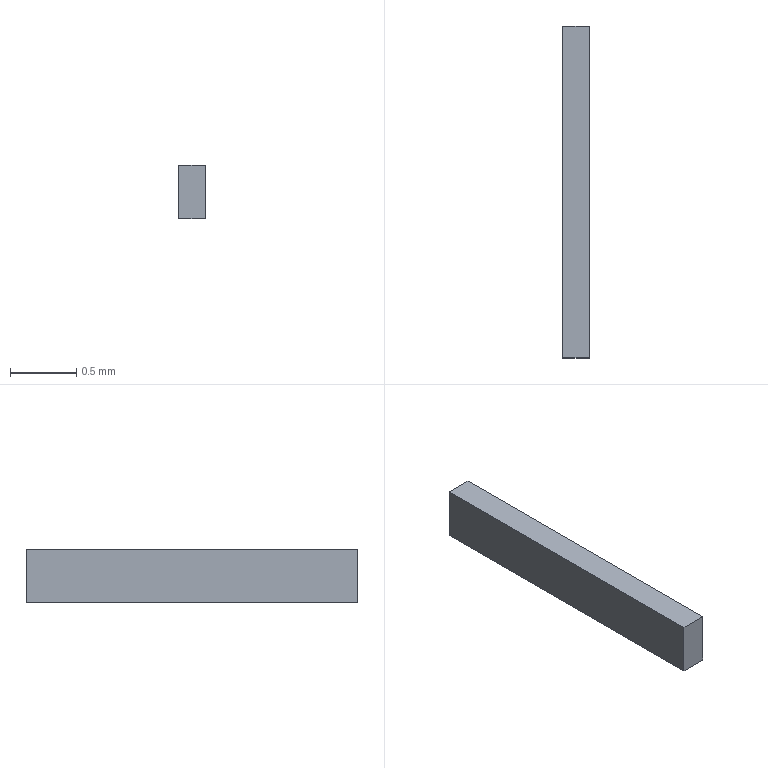Part | STEP file | RJ-USIO-V1_2-220411_74 | 1 solid | 6 faces | box 0.2 x 2.5 x 0.4 mm | volume 0.2 mm3 | plane 6
STEP:
#1=CARTESIAN_POINT('',(0.,0.,0.));
#2=DIRECTION('',(0.,0.,1.));
#3=DIRECTION('',(1.,0.,0.));
#4=AXIS2_PLACEMENT_3D('',#1,#2,#3);
#5=CARTESIAN_POINT('',(43.7,30.6,0.4));
#6=VERTEX_POINT('',#5);
#7=CARTESIAN_POINT('',(43.7,28.1,0.4));
#8=VERTEX_POINT('',#7);
#9=CARTESIAN_POINT('',(43.7,30.6,0.4));
#10=DIRECTION('',(0.,-1.,0.));
#11=VECTOR('',#10,1.);
#12=LINE('',#9,#11);
#13=CARTESIAN_POINT('',(43.7,28.1,0.4));
#14=DIRECTION('',(0.,0.,-1.));
#15=DIRECTION('',(1.,0.,0.));
#16=AXIS2_PLACEMENT_3D('',#13,#14,#15);
#17=PLANE('',#16);
#18=CARTESIAN_POINT('',(0.,-2.5));
#19=DIRECTION('',(0.,1.));
#20=VECTOR('',#19,1.);
#21=LINE('',#18,#20);
#22=(GEOMETRIC_REPRESENTATION_CONTEXT(2)PARAMETRIC_REPRESENTATION_CONTEXT()REPRESENTATION_CONTEXT('',''));
#23=DEFINITIONAL_REPRESENTATION('',(#21),#22);
#24=PCURVE('',#17,#23);
#25=CARTESIAN_POINT('',(43.7,28.1,0.));
#26=DIRECTION('',(-1.,0.,0.));
#27=DIRECTION('',(0.,-1.,0.));
#28=AXIS2_PLACEMENT_3D('',#25,#26,#27);
#29=PLANE('',#28);
#30=CARTESIAN_POINT('',(-2.5,0.4));
#31=DIRECTION('',(1.,0.));
#32=VECTOR('',#31,1.);
#33=LINE('',#30,#32);
#34=(GEOMETRIC_REPRESENTATION_CONTEXT(2)PARAMETRIC_REPRESENTATION_CONTEXT()REPRESENTATION_CONTEXT('',''));
#35=DEFINITIONAL_REPRESENTATION('',(#33),#34);
#36=PCURVE('',#29,#35);
#37=SURFACE_CURVE('',#12,(#24,#36),.PCURVE_S1.);
#38=EDGE_CURVE('',#6,#8,#37,.T.);
#39=ORIENTED_EDGE('',*,*,#38,.T.);
#40=CARTESIAN_POINT('',(43.5,28.1,0.4));
#41=VERTEX_POINT('',#40);
#42=CARTESIAN_POINT('',(43.7,28.1,0.4));
#43=DIRECTION('',(-1.,0.,0.));
#44=VECTOR('',#43,1.);
#45=LINE('',#42,#44);
#46=CARTESIAN_POINT('',(0.,0.));
#47=DIRECTION('',(-1.,0.));
#48=VECTOR('',#47,1.);
#49=LINE('',#46,#48);
#50=(GEOMETRIC_REPRESENTATION_CONTEXT(2)PARAMETRIC_REPRESENTATION_CONTEXT()REPRESENTATION_CONTEXT('',''));
#51=DEFINITIONAL_REPRESENTATION('',(#49),#50);
#52=PCURVE('',#17,#51);
#53=CARTESIAN_POINT('',(43.5,28.1,0.));
#54=DIRECTION('',(0.,1.,0.));
#55=DIRECTION('',(-1.,0.,0.));
#56=AXIS2_PLACEMENT_3D('',#53,#54,#55);
#57=PLANE('',#56);
#58=CARTESIAN_POINT('',(-0.2,0.4));
#59=DIRECTION('',(1.,0.));
#60=VECTOR('',#59,1.);
#61=LINE('',#58,#60);
#62=(GEOMETRIC_REPRESENTATION_CONTEXT(2)PARAMETRIC_REPRESENTATION_CONTEXT()REPRESENTATION_CONTEXT('',''));
#63=DEFINITIONAL_REPRESENTATION('',(#61),#62);
#64=PCURVE('',#57,#63);
#65=SURFACE_CURVE('',#45,(#52,#64),.PCURVE_S1.);
#66=EDGE_CURVE('',#8,#41,#65,.T.);
#67=ORIENTED_EDGE('',*,*,#66,.T.);
#68=CARTESIAN_POINT('',(43.5,30.6,0.4));
#69=VERTEX_POINT('',#68);
#70=CARTESIAN_POINT('',(43.5,28.1,0.4));
#71=DIRECTION('',(0.,1.,0.));
#72=VECTOR('',#71,1.);
#73=LINE('',#70,#72);
#74=CARTESIAN_POINT('',(-0.2,0.));
#75=DIRECTION('',(0.,-1.));
#76=VECTOR('',#75,1.);
#77=LINE('',#74,#76);
#78=(GEOMETRIC_REPRESENTATION_CONTEXT(2)PARAMETRIC_REPRESENTATION_CONTEXT()REPRESENTATION_CONTEXT('',''));
#79=DEFINITIONAL_REPRESENTATION('',(#77),#78);
#80=PCURVE('',#17,#79);
#81=CARTESIAN_POINT('',(43.5,30.6,0.));
#82=DIRECTION('',(1.,0.,0.));
#83=DIRECTION('',(0.,1.,0.));
#84=AXIS2_PLACEMENT_3D('',#81,#82,#83);
#85=PLANE('',#84);
#86=CARTESIAN_POINT('',(-2.5,0.4));
#87=DIRECTION('',(1.,0.));
#88=VECTOR('',#87,1.);
#89=LINE('',#86,#88);
#90=(GEOMETRIC_REPRESENTATION_CONTEXT(2)PARAMETRIC_REPRESENTATION_CONTEXT()REPRESENTATION_CONTEXT('',''));
#91=DEFINITIONAL_REPRESENTATION('',(#89),#90);
#92=PCURVE('',#85,#91);
#93=SURFACE_CURVE('',#73,(#80,#92),.PCURVE_S1.);
#94=EDGE_CURVE('',#41,#69,#93,.T.);
#95=ORIENTED_EDGE('',*,*,#94,.T.);
#96=CARTESIAN_POINT('',(43.5,30.6,0.4));
#97=DIRECTION('',(1.,0.,0.));
#98=VECTOR('',#97,1.);
#99=LINE('',#96,#98);
#100=CARTESIAN_POINT('',(-0.2,-2.5));
#101=DIRECTION('',(1.,0.));
#102=VECTOR('',#101,1.);
#103=LINE('',#100,#102);
#104=(GEOMETRIC_REPRESENTATION_CONTEXT(2)PARAMETRIC_REPRESENTATION_CONTEXT()REPRESENTATION_CONTEXT('',''));
#105=DEFINITIONAL_REPRESENTATION('',(#103),#104);
#106=PCURVE('',#17,#105);
#107=CARTESIAN_POINT('',(43.7,30.6,0.));
#108=DIRECTION('',(0.,-1.,0.));
#109=DIRECTION('',(1.,0.,0.));
#110=AXIS2_PLACEMENT_3D('',#107,#108,#109);
#111=PLANE('',#110);
#112=CARTESIAN_POINT('',(-0.2,0.4));
#113=DIRECTION('',(1.,0.));
#114=VECTOR('',#113,1.);
#115=LINE('',#112,#114);
#116=(GEOMETRIC_REPRESENTATION_CONTEXT(2)PARAMETRIC_REPRESENTATION_CONTEXT()REPRESENTATION_CONTEXT('',''));
#117=DEFINITIONAL_REPRESENTATION('',(#115),#116);
#118=PCURVE('',#111,#117);
#119=SURFACE_CURVE('',#99,(#106,#118),.PCURVE_S1.);
#120=EDGE_CURVE('',#69,#6,#119,.T.);
#121=ORIENTED_EDGE('',*,*,#120,.T.);
#122=EDGE_LOOP('',(#39,#67,#95,#121));
#123=FACE_BOUND('',#122,.F.);
#124=ADVANCED_FACE('',(#123),#17,.F.);
#125=CARTESIAN_POINT('',(43.7,30.6,0.));
#126=VERTEX_POINT('',#125);
#127=CARTESIAN_POINT('',(43.7,28.1,0.));
#128=VERTEX_POINT('',#127);
#129=CARTESIAN_POINT('',(43.7,30.6,0.));
#130=DIRECTION('',(0.,-1.,0.));
#131=VECTOR('',#130,1.);
#132=LINE('',#129,#131);
#133=CARTESIAN_POINT('',(-2.5,0.));
#134=DIRECTION('',(1.,0.));
#135=VECTOR('',#134,1.);
#136=LINE('',#133,#135);
#137=(GEOMETRIC_REPRESENTATION_CONTEXT(2)PARAMETRIC_REPRESENTATION_CONTEXT()REPRESENTATION_CONTEXT('',''));
#138=DEFINITIONAL_REPRESENTATION('',(#136),#137);
#139=PCURVE('',#29,#138);
#140=CARTESIAN_POINT('',(43.7,28.1,0.));
#141=DIRECTION('',(0.,0.,-1.));
#142=DIRECTION('',(1.,0.,0.));
#143=AXIS2_PLACEMENT_3D('',#140,#141,#142);
#144=PLANE('',#143);
#145=CARTESIAN_POINT('',(0.,-2.5));
#146=DIRECTION('',(0.,1.));
#147=VECTOR('',#146,1.);
#148=LINE('',#145,#147);
#149=(GEOMETRIC_REPRESENTATION_CONTEXT(2)PARAMETRIC_REPRESENTATION_CONTEXT()REPRESENTATION_CONTEXT('',''));
#150=DEFINITIONAL_REPRESENTATION('',(#148),#149);
#151=PCURVE('',#144,#150);
#152=SURFACE_CURVE('',#132,(#139,#151),.PCURVE_S1.);
#153=EDGE_CURVE('',#126,#128,#152,.T.);
#154=ORIENTED_EDGE('',*,*,#153,.T.);
#155=CARTESIAN_POINT('',(43.7,28.1,0.4));
#156=DIRECTION('',(0.,0.,-1.));
#157=VECTOR('',#156,1.);
#158=LINE('',#155,#157);
#159=CARTESIAN_POINT('',(0.,0.4));
#160=DIRECTION('',(0.,-1.));
#161=VECTOR('',#160,1.);
#162=LINE('',#159,#161);
#163=(GEOMETRIC_REPRESENTATION_CONTEXT(2)PARAMETRIC_REPRESENTATION_CONTEXT()REPRESENTATION_CONTEXT('',''));
#164=DEFINITIONAL_REPRESENTATION('',(#162),#163);
#165=PCURVE('',#29,#164);
#166=CARTESIAN_POINT('',(-0.2,0.4));
#167=DIRECTION('',(0.,-1.));
#168=VECTOR('',#167,1.);
#169=LINE('',#166,#168);
#170=(GEOMETRIC_REPRESENTATION_CONTEXT(2)PARAMETRIC_REPRESENTATION_CONTEXT()REPRESENTATION_CONTEXT('',''));
#171=DEFINITIONAL_REPRESENTATION('',(#169),#170);
#172=PCURVE('',#57,#171);
#173=SURFACE_CURVE('',#158,(#165,#172),.PCURVE_S1.);
#174=EDGE_CURVE('',#8,#128,#173,.T.);
#175=ORIENTED_EDGE('',*,*,#174,.F.);
#176=ORIENTED_EDGE('',*,*,#38,.F.);
#177=CARTESIAN_POINT('',(43.7,30.6,0.4));
#178=DIRECTION('',(0.,0.,-1.));
#179=VECTOR('',#178,1.);
#180=LINE('',#177,#179);
#181=CARTESIAN_POINT('',(-2.5,0.4));
#182=DIRECTION('',(0.,-1.));
#183=VECTOR('',#182,1.);
#184=LINE('',#181,#183);
#185=(GEOMETRIC_REPRESENTATION_CONTEXT(2)PARAMETRIC_REPRESENTATION_CONTEXT()REPRESENTATION_CONTEXT('',''));
#186=DEFINITIONAL_REPRESENTATION('',(#184),#185);
#187=PCURVE('',#29,#186);
#188=CARTESIAN_POINT('',(0.,0.4));
#189=DIRECTION('',(0.,-1.));
#190=VECTOR('',#189,1.);
#191=LINE('',#188,#190);
#192=(GEOMETRIC_REPRESENTATION_CONTEXT(2)PARAMETRIC_REPRESENTATION_CONTEXT()REPRESENTATION_CONTEXT('',''));
#193=DEFINITIONAL_REPRESENTATION('',(#191),#192);
#194=PCURVE('',#111,#193);
#195=SURFACE_CURVE('',#180,(#187,#194),.PCURVE_S1.);
#196=EDGE_CURVE('',#6,#126,#195,.T.);
#197=ORIENTED_EDGE('',*,*,#196,.T.);
#198=EDGE_LOOP('',(#154,#175,#176,#197));
#199=FACE_BOUND('',#198,.F.);
#200=ADVANCED_FACE('',(#199),#29,.F.);
#201=CARTESIAN_POINT('',(43.5,28.1,0.));
#202=VERTEX_POINT('',#201);
#203=CARTESIAN_POINT('',(43.7,28.1,0.));
#204=DIRECTION('',(-1.,0.,0.));
#205=VECTOR('',#204,1.);
#206=LINE('',#203,#205);
#207=CARTESIAN_POINT('',(0.,0.));
#208=DIRECTION('',(-1.,0.));
#209=VECTOR('',#208,1.);
#210=LINE('',#207,#209);
#211=(GEOMETRIC_REPRESENTATION_CONTEXT(2)PARAMETRIC_REPRESENTATION_CONTEXT()REPRESENTATION_CONTEXT('',''));
#212=DEFINITIONAL_REPRESENTATION('',(#210),#211);
#213=PCURVE('',#144,#212);
#214=CARTESIAN_POINT('',(-0.2,0.));
#215=DIRECTION('',(1.,0.));
#216=VECTOR('',#215,1.);
#217=LINE('',#214,#216);
#218=(GEOMETRIC_REPRESENTATION_CONTEXT(2)PARAMETRIC_REPRESENTATION_CONTEXT()REPRESENTATION_CONTEXT('',''));
#219=DEFINITIONAL_REPRESENTATION('',(#217),#218);
#220=PCURVE('',#57,#219);
#221=SURFACE_CURVE('',#206,(#213,#220),.PCURVE_S1.);
#222=EDGE_CURVE('',#128,#202,#221,.T.);
#223=ORIENTED_EDGE('',*,*,#222,.F.);
#224=ORIENTED_EDGE('',*,*,#153,.F.);
#225=CARTESIAN_POINT('',(43.5,30.6,0.));
#226=VERTEX_POINT('',#225);
#227=CARTESIAN_POINT('',(43.5,30.6,0.));
#228=DIRECTION('',(1.,0.,0.));
#229=VECTOR('',#228,1.);
#230=LINE('',#227,#229);
#231=CARTESIAN_POINT('',(-0.2,-2.5));
#232=DIRECTION('',(1.,0.));
#233=VECTOR('',#232,1.);
#234=LINE('',#231,#233);
#235=(GEOMETRIC_REPRESENTATION_CONTEXT(2)PARAMETRIC_REPRESENTATION_CONTEXT()REPRESENTATION_CONTEXT('',''));
#236=DEFINITIONAL_REPRESENTATION('',(#234),#235);
#237=PCURVE('',#144,#236);
#238=CARTESIAN_POINT('',(-0.2,0.));
#239=DIRECTION('',(1.,0.));
#240=VECTOR('',#239,1.);
#241=LINE('',#238,#240);
#242=(GEOMETRIC_REPRESENTATION_CONTEXT(2)PARAMETRIC_REPRESENTATION_CONTEXT()REPRESENTATION_CONTEXT('',''));
#243=DEFINITIONAL_REPRESENTATION('',(#241),#242);
#244=PCURVE('',#111,#243);
#245=SURFACE_CURVE('',#230,(#237,#244),.PCURVE_S1.);
#246=EDGE_CURVE('',#226,#126,#245,.T.);
#247=ORIENTED_EDGE('',*,*,#246,.F.);
#248=CARTESIAN_POINT('',(43.5,28.1,0.));
#249=DIRECTION('',(0.,1.,0.));
#250=VECTOR('',#249,1.);
#251=LINE('',#248,#250);
#252=CARTESIAN_POINT('',(-0.2,0.));
#253=DIRECTION('',(0.,-1.));
#254=VECTOR('',#253,1.);
#255=LINE('',#252,#254);
#256=(GEOMETRIC_REPRESENTATION_CONTEXT(2)PARAMETRIC_REPRESENTATION_CONTEXT()REPRESENTATION_CONTEXT('',''));
#257=DEFINITIONAL_REPRESENTATION('',(#255),#256);
#258=PCURVE('',#144,#257);
#259=CARTESIAN_POINT('',(-2.5,0.));
#260=DIRECTION('',(1.,0.));
#261=VECTOR('',#260,1.);
#262=LINE('',#259,#261);
#263=(GEOMETRIC_REPRESENTATION_CONTEXT(2)PARAMETRIC_REPRESENTATION_CONTEXT()REPRESENTATION_CONTEXT('',''));
#264=DEFINITIONAL_REPRESENTATION('',(#262),#263);
#265=PCURVE('',#85,#264);
#266=SURFACE_CURVE('',#251,(#258,#265),.PCURVE_S1.);
#267=EDGE_CURVE('',#202,#226,#266,.T.);
#268=ORIENTED_EDGE('',*,*,#267,.F.);
#269=EDGE_LOOP('',(#223,#224,#247,#268));
#270=FACE_BOUND('',#269,.F.);
#271=ADVANCED_FACE('',(#270),#144,.T.);
#272=ORIENTED_EDGE('',*,*,#222,.T.);
#273=CARTESIAN_POINT('',(43.5,28.1,0.4));
#274=DIRECTION('',(0.,0.,-1.));
#275=VECTOR('',#274,1.);
#276=LINE('',#273,#275);
#277=CARTESIAN_POINT('',(0.,0.4));
#278=DIRECTION('',(0.,-1.));
#279=VECTOR('',#278,1.);
#280=LINE('',#277,#279);
#281=(GEOMETRIC_REPRESENTATION_CONTEXT(2)PARAMETRIC_REPRESENTATION_CONTEXT()REPRESENTATION_CONTEXT('',''));
#282=DEFINITIONAL_REPRESENTATION('',(#280),#281);
#283=PCURVE('',#57,#282);
#284=CARTESIAN_POINT('',(-2.5,0.4));
#285=DIRECTION('',(0.,-1.));
#286=VECTOR('',#285,1.);
#287=LINE('',#284,#286);
#288=(GEOMETRIC_REPRESENTATION_CONTEXT(2)PARAMETRIC_REPRESENTATION_CONTEXT()REPRESENTATION_CONTEXT('',''));
#289=DEFINITIONAL_REPRESENTATION('',(#287),#288);
#290=PCURVE('',#85,#289);
#291=SURFACE_CURVE('',#276,(#283,#290),.PCURVE_S1.);
#292=EDGE_CURVE('',#41,#202,#291,.T.);
#293=ORIENTED_EDGE('',*,*,#292,.F.);
#294=ORIENTED_EDGE('',*,*,#66,.F.);
#295=ORIENTED_EDGE('',*,*,#174,.T.);
#296=EDGE_LOOP('',(#272,#293,#294,#295));
#297=FACE_BOUND('',#296,.F.);
#298=ADVANCED_FACE('',(#297),#57,.F.);
#299=ORIENTED_EDGE('',*,*,#267,.T.);
#300=CARTESIAN_POINT('',(43.5,30.6,0.4));
#301=DIRECTION('',(0.,0.,-1.));
#302=VECTOR('',#301,1.);
#303=LINE('',#300,#302);
#304=CARTESIAN_POINT('',(0.,0.4));
#305=DIRECTION('',(0.,-1.));
#306=VECTOR('',#305,1.);
#307=LINE('',#304,#306);
#308=(GEOMETRIC_REPRESENTATION_CONTEXT(2)PARAMETRIC_REPRESENTATION_CONTEXT()REPRESENTATION_CONTEXT('',''));
#309=DEFINITIONAL_REPRESENTATION('',(#307),#308);
#310=PCURVE('',#85,#309);
#311=CARTESIAN_POINT('',(-0.2,0.4));
#312=DIRECTION('',(0.,-1.));
#313=VECTOR('',#312,1.);
#314=LINE('',#311,#313);
#315=(GEOMETRIC_REPRESENTATION_CONTEXT(2)PARAMETRIC_REPRESENTATION_CONTEXT()REPRESENTATION_CONTEXT('',''));
#316=DEFINITIONAL_REPRESENTATION('',(#314),#315);
#317=PCURVE('',#111,#316);
#318=SURFACE_CURVE('',#303,(#310,#317),.PCURVE_S1.);
#319=EDGE_CURVE('',#69,#226,#318,.T.);
#320=ORIENTED_EDGE('',*,*,#319,.F.);
#321=ORIENTED_EDGE('',*,*,#94,.F.);
#322=ORIENTED_EDGE('',*,*,#292,.T.);
#323=EDGE_LOOP('',(#299,#320,#321,#322));
#324=FACE_BOUND('',#323,.F.);
#325=ADVANCED_FACE('',(#324),#85,.F.);
#326=ORIENTED_EDGE('',*,*,#246,.T.);
#327=ORIENTED_EDGE('',*,*,#196,.F.);
#328=ORIENTED_EDGE('',*,*,#120,.F.);
#329=ORIENTED_EDGE('',*,*,#319,.T.);
#330=EDGE_LOOP('',(#326,#327,#328,#329));
#331=FACE_BOUND('',#330,.F.);
#332=ADVANCED_FACE('',(#331),#111,.F.);
#333=CLOSED_SHELL('',(#124,#200,#271,#298,#325,#332));
#334=MANIFOLD_SOLID_BREP('',#333);
#335=(LENGTH_UNIT()NAMED_UNIT(*)SI_UNIT(.MILLI.,.METRE.));
#336=UNCERTAINTY_MEASURE_WITH_UNIT(LENGTH_MEASURE(0.0000001),#335,'','');
#337=(NAMED_UNIT(*)PLANE_ANGLE_UNIT()SI_UNIT($,.RADIAN.));
#338=(NAMED_UNIT(*)SI_UNIT($,.STERADIAN.)SOLID_ANGLE_UNIT());
#339=(GEOMETRIC_REPRESENTATION_CONTEXT(3)GLOBAL_UNCERTAINTY_ASSIGNED_CONTEXT((#336))GLOBAL_UNIT_ASSIGNED_CONTEXT((#335,#337,#338))REPRESENTATION_CONTEXT('',''));
#340=ADVANCED_BREP_SHAPE_REPRESENTATION('',(#4,#334),#339);